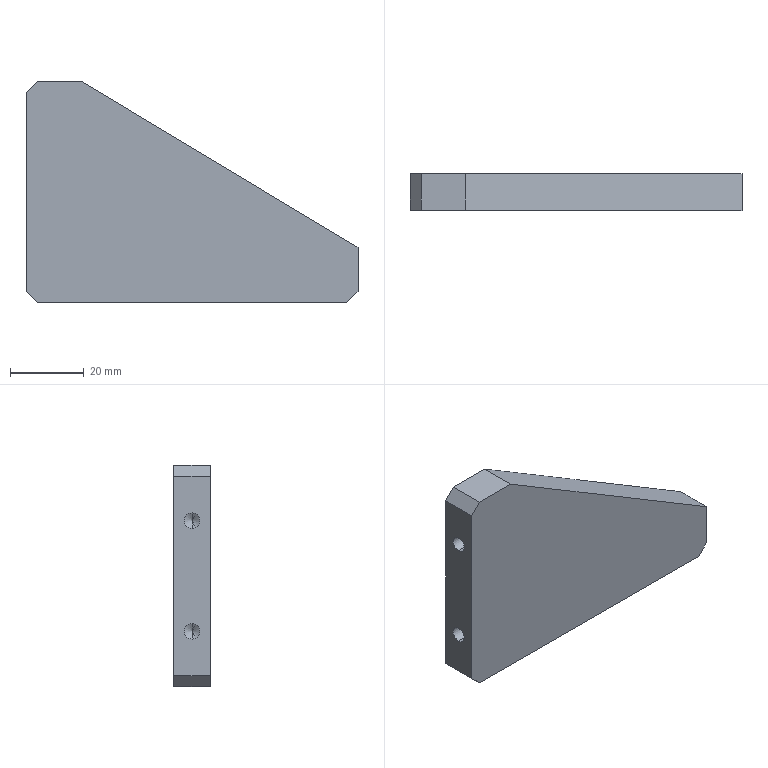Part | SolidWorks | features HoleWzd 2, Chamfer 1, Extrusion 1, ICE 1 | 1 solid | 30 faces | box 90 x 10 x 60 mm | volume 36102 mm3 | cylinder 10 | cone 10 | plane 10 | commonest cylinder face diameters 4.2 x10
STEP:
#1=CARTESIAN_POINT('',(-27.9,5.,-17.6));
#2=VERTEX_POINT('',#1);
#3=CARTESIAN_POINT('',(-32.1,5.,-17.6));
#4=VERTEX_POINT('',#3);
#5=CARTESIAN_POINT('',(-30.,5.,-17.6));
#6=DIRECTION('',(0.,0.,-1.));
#7=DIRECTION('',(-1.,0.,0.));
#8=AXIS2_PLACEMENT_3D('',#5,#6,#7);
#9=CIRCLE('',#8,2.1);
#10=EDGE_CURVE('',#2,#4,#9,.T.);
#11=ORIENTED_EDGE('',*,*,#10,.F.);
#12=CARTESIAN_POINT('',(-27.9,5.,-30.));
#13=VERTEX_POINT('',#12);
#14=CARTESIAN_POINT('',(-27.9,5.,-30.));
#15=DIRECTION('',(0.,0.,-1.));
#16=VECTOR('',#15,1000.);
#17=LINE('',#14,#16);
#18=EDGE_CURVE('',#2,#13,#17,.T.);
#19=ORIENTED_EDGE('',*,*,#18,.T.);
#20=CARTESIAN_POINT('',(-32.1,5.,-30.));
#21=VERTEX_POINT('',#20);
#22=CARTESIAN_POINT('',(-30.,5.,-30.));
#23=DIRECTION('',(0.,0.,-1.));
#24=DIRECTION('',(-1.,0.,0.));
#25=AXIS2_PLACEMENT_3D('',#22,#23,#24);
#26=CIRCLE('',#25,2.1);
#27=EDGE_CURVE('',#13,#21,#26,.T.);
#28=ORIENTED_EDGE('',*,*,#27,.T.);
#29=CARTESIAN_POINT('',(-32.1,5.,-30.));
#30=DIRECTION('',(0.,0.,-1.));
#31=VECTOR('',#30,1000.);
#32=LINE('',#29,#31);
#33=EDGE_CURVE('',#4,#21,#32,.T.);
#34=ORIENTED_EDGE('',*,*,#33,.F.);
#35=EDGE_LOOP('',(#11,#19,#28,#34));
#36=FACE_OUTER_BOUND('',#35,.T.);
#37=CARTESIAN_POINT('',(-30.,5.,-30.));
#38=DIRECTION('',(0.,0.,-1.));
#39=DIRECTION('',(-1.,0.,0.));
#40=AXIS2_PLACEMENT_3D('',#37,#38,#39);
#41=CYLINDRICAL_SURFACE('',#40,2.1);
#42=ADVANCED_FACE('',(#36),#41,.F.);
#43=CARTESIAN_POINT('',(-30.,5.,-16.338));
#44=VERTEX_POINT('',#43);
#45=CARTESIAN_POINT('',(-32.1,5.,-17.6));
#46=DIRECTION('',(-0.8572,0.,-0.515));
#47=VECTOR('',#46,1000.);
#48=LINE('',#45,#47);
#49=EDGE_CURVE('',#44,#4,#48,.T.);
#50=ORIENTED_EDGE('',*,*,#49,.F.);
#51=CARTESIAN_POINT('',(-27.9,5.,-17.6));
#52=DIRECTION('',(0.8572,0.,-0.515));
#53=VECTOR('',#52,1000.);
#54=LINE('',#51,#53);
#55=EDGE_CURVE('',#44,#2,#54,.T.);
#56=ORIENTED_EDGE('',*,*,#55,.T.);
#57=ORIENTED_EDGE('',*,*,#10,.T.);
#58=EDGE_LOOP('',(#50,#56,#57));
#59=FACE_OUTER_BOUND('',#58,.T.);
#60=CARTESIAN_POINT('',(-30.,5.,-17.6));
#61=DIRECTION('',(0.,0.,-1.));
#62=DIRECTION('',(-1.,0.,0.));
#63=AXIS2_PLACEMENT_3D('',#60,#61,#62);
#64=CONICAL_SURFACE('',#63,2.1,1.03);
#65=ADVANCED_FACE('',(#59),#64,.F.);
#66=CARTESIAN_POINT('',(2.1,5.,-17.6));
#67=VERTEX_POINT('',#66);
#68=CARTESIAN_POINT('',(-2.1,5.,-17.6));
#69=VERTEX_POINT('',#68);
#70=CARTESIAN_POINT('',(0.,5.,-17.6));
#71=DIRECTION('',(0.,0.,-1.));
#72=DIRECTION('',(-1.,0.,0.));
#73=AXIS2_PLACEMENT_3D('',#70,#71,#72);
#74=CIRCLE('',#73,2.1);
#75=EDGE_CURVE('',#67,#69,#74,.T.);
#76=ORIENTED_EDGE('',*,*,#75,.F.);
#77=CARTESIAN_POINT('',(2.1,5.,-30.));
#78=VERTEX_POINT('',#77);
#79=CARTESIAN_POINT('',(2.1,5.,-30.));
#80=DIRECTION('',(0.,0.,-1.));
#81=VECTOR('',#80,1000.);
#82=LINE('',#79,#81);
#83=EDGE_CURVE('',#67,#78,#82,.T.);
#84=ORIENTED_EDGE('',*,*,#83,.T.);
#85=CARTESIAN_POINT('',(-2.1,5.,-30.));
#86=VERTEX_POINT('',#85);
#87=CARTESIAN_POINT('',(0.,5.,-30.));
#88=DIRECTION('',(0.,0.,-1.));
#89=DIRECTION('',(-1.,0.,0.));
#90=AXIS2_PLACEMENT_3D('',#87,#88,#89);
#91=CIRCLE('',#90,2.1);
#92=EDGE_CURVE('',#78,#86,#91,.T.);
#93=ORIENTED_EDGE('',*,*,#92,.T.);
#94=CARTESIAN_POINT('',(-2.1,5.,-30.));
#95=DIRECTION('',(0.,0.,-1.));
#96=VECTOR('',#95,1000.);
#97=LINE('',#94,#96);
#98=EDGE_CURVE('',#69,#86,#97,.T.);
#99=ORIENTED_EDGE('',*,*,#98,.F.);
#100=EDGE_LOOP('',(#76,#84,#93,#99));
#101=FACE_OUTER_BOUND('',#100,.T.);
#102=CARTESIAN_POINT('',(0.,5.,-30.));
#103=DIRECTION('',(0.,0.,-1.));
#104=DIRECTION('',(-1.,0.,0.));
#105=AXIS2_PLACEMENT_3D('',#102,#103,#104);
#106=CYLINDRICAL_SURFACE('',#105,2.1);
#107=ADVANCED_FACE('',(#101),#106,.F.);
#108=CARTESIAN_POINT('',(0.,5.,-16.338));
#109=VERTEX_POINT('',#108);
#110=CARTESIAN_POINT('',(-2.1,5.,-17.6));
#111=DIRECTION('',(-0.8572,0.,-0.515));
#112=VECTOR('',#111,1000.);
#113=LINE('',#110,#112);
#114=EDGE_CURVE('',#109,#69,#113,.T.);
#115=ORIENTED_EDGE('',*,*,#114,.F.);
#116=CARTESIAN_POINT('',(2.1,5.,-17.6));
#117=DIRECTION('',(0.8572,0.,-0.515));
#118=VECTOR('',#117,1000.);
#119=LINE('',#116,#118);
#120=EDGE_CURVE('',#109,#67,#119,.T.);
#121=ORIENTED_EDGE('',*,*,#120,.T.);
#122=ORIENTED_EDGE('',*,*,#75,.T.);
#123=EDGE_LOOP('',(#115,#121,#122));
#124=FACE_OUTER_BOUND('',#123,.T.);
#125=CARTESIAN_POINT('',(0.,5.,-17.6));
#126=DIRECTION('',(0.,0.,-1.));
#127=DIRECTION('',(-1.,0.,0.));
#128=AXIS2_PLACEMENT_3D('',#125,#126,#127);
#129=CONICAL_SURFACE('',#128,2.1,1.03);
#130=ADVANCED_FACE('',(#124),#129,.F.);
#131=CARTESIAN_POINT('',(32.1,5.,-17.6));
#132=VERTEX_POINT('',#131);
#133=CARTESIAN_POINT('',(27.9,5.,-17.6));
#134=VERTEX_POINT('',#133);
#135=CARTESIAN_POINT('',(30.,5.,-17.6));
#136=DIRECTION('',(0.,0.,-1.));
#137=DIRECTION('',(-1.,0.,0.));
#138=AXIS2_PLACEMENT_3D('',#135,#136,#137);
#139=CIRCLE('',#138,2.1);
#140=EDGE_CURVE('',#132,#134,#139,.T.);
#141=ORIENTED_EDGE('',*,*,#140,.F.);
#142=CARTESIAN_POINT('',(32.1,5.,-30.));
#143=VERTEX_POINT('',#142);
#144=CARTESIAN_POINT('',(32.1,5.,-30.));
#145=DIRECTION('',(0.,0.,-1.));
#146=VECTOR('',#145,1000.);
#147=LINE('',#144,#146);
#148=EDGE_CURVE('',#132,#143,#147,.T.);
#149=ORIENTED_EDGE('',*,*,#148,.T.);
#150=CARTESIAN_POINT('',(27.9,5.,-30.));
#151=VERTEX_POINT('',#150);
#152=CARTESIAN_POINT('',(30.,5.,-30.));
#153=DIRECTION('',(0.,0.,-1.));
#154=DIRECTION('',(-1.,0.,0.));
#155=AXIS2_PLACEMENT_3D('',#152,#153,#154);
#156=CIRCLE('',#155,2.1);
#157=EDGE_CURVE('',#143,#151,#156,.T.);
#158=ORIENTED_EDGE('',*,*,#157,.T.);
#159=CARTESIAN_POINT('',(27.9,5.,-30.));
#160=DIRECTION('',(0.,0.,-1.));
#161=VECTOR('',#160,1000.);
#162=LINE('',#159,#161);
#163=EDGE_CURVE('',#134,#151,#162,.T.);
#164=ORIENTED_EDGE('',*,*,#163,.F.);
#165=EDGE_LOOP('',(#141,#149,#158,#164));
#166=FACE_OUTER_BOUND('',#165,.T.);
#167=CARTESIAN_POINT('',(30.,5.,-30.));
#168=DIRECTION('',(0.,0.,-1.));
#169=DIRECTION('',(-1.,0.,0.));
#170=AXIS2_PLACEMENT_3D('',#167,#168,#169);
#171=CYLINDRICAL_SURFACE('',#170,2.1);
#172=ADVANCED_FACE('',(#166),#171,.F.);
#173=CARTESIAN_POINT('',(30.,5.,-16.338));
#174=VERTEX_POINT('',#173);
#175=CARTESIAN_POINT('',(27.9,5.,-17.6));
#176=DIRECTION('',(-0.8572,0.,-0.515));
#177=VECTOR('',#176,1000.);
#178=LINE('',#175,#177);
#179=EDGE_CURVE('',#174,#134,#178,.T.);
#180=ORIENTED_EDGE('',*,*,#179,.F.);
#181=CARTESIAN_POINT('',(32.1,5.,-17.6));
#182=DIRECTION('',(0.8572,0.,-0.515));
#183=VECTOR('',#182,1000.);
#184=LINE('',#181,#183);
#185=EDGE_CURVE('',#174,#132,#184,.T.);
#186=ORIENTED_EDGE('',*,*,#185,.T.);
#187=ORIENTED_EDGE('',*,*,#140,.T.);
#188=EDGE_LOOP('',(#180,#186,#187));
#189=FACE_OUTER_BOUND('',#188,.T.);
#190=CARTESIAN_POINT('',(30.,5.,-17.6));
#191=DIRECTION('',(0.,0.,-1.));
#192=DIRECTION('',(-1.,0.,0.));
#193=AXIS2_PLACEMENT_3D('',#190,#191,#192);
#194=CONICAL_SURFACE('',#193,2.1,1.03);
#195=ADVANCED_FACE('',(#189),#194,.F.);
#196=CARTESIAN_POINT('',(-32.6,5.,-17.1));
#197=VERTEX_POINT('',#196);
#198=CARTESIAN_POINT('',(-32.6,5.,-12.9));
#199=VERTEX_POINT('',#198);
#200=CARTESIAN_POINT('',(-32.6,5.,-15.));
#201=DIRECTION('',(-1.,0.,0.));
#202=DIRECTION('',(0.,0.,1.));
#203=AXIS2_PLACEMENT_3D('',#200,#201,#202);
#204=CIRCLE('',#203,2.1);
#205=EDGE_CURVE('',#197,#199,#204,.T.);
#206=ORIENTED_EDGE('',*,*,#205,.F.);
#207=CARTESIAN_POINT('',(-45.,5.,-17.1));
#208=VERTEX_POINT('',#207);
#209=CARTESIAN_POINT('',(-45.,5.,-17.1));
#210=DIRECTION('',(-1.,0.,0.));
#211=VECTOR('',#210,1000.);
#212=LINE('',#209,#211);
#213=EDGE_CURVE('',#197,#208,#212,.T.);
#214=ORIENTED_EDGE('',*,*,#213,.T.);
#215=CARTESIAN_POINT('',(-45.,5.,-12.9));
#216=VERTEX_POINT('',#215);
#217=CARTESIAN_POINT('',(-45.,5.,-15.));
#218=DIRECTION('',(-1.,0.,0.));
#219=DIRECTION('',(0.,0.,1.));
#220=AXIS2_PLACEMENT_3D('',#217,#218,#219);
#221=CIRCLE('',#220,2.1);
#222=EDGE_CURVE('',#208,#216,#221,.T.);
#223=ORIENTED_EDGE('',*,*,#222,.T.);
#224=CARTESIAN_POINT('',(-45.,5.,-12.9));
#225=DIRECTION('',(-1.,0.,0.));
#226=VECTOR('',#225,1000.);
#227=LINE('',#224,#226);
#228=EDGE_CURVE('',#199,#216,#227,.T.);
#229=ORIENTED_EDGE('',*,*,#228,.F.);
#230=EDGE_LOOP('',(#206,#214,#223,#229));
#231=FACE_OUTER_BOUND('',#230,.T.);
#232=CARTESIAN_POINT('',(-45.,5.,-15.));
#233=DIRECTION('',(-1.,0.,0.));
#234=DIRECTION('',(0.,0.,1.));
#235=AXIS2_PLACEMENT_3D('',#232,#233,#234);
#236=CYLINDRICAL_SURFACE('',#235,2.1);
#237=ADVANCED_FACE('',(#231),#236,.F.);
#238=CARTESIAN_POINT('',(-31.338,5.,-15.));
#239=VERTEX_POINT('',#238);
#240=CARTESIAN_POINT('',(-32.6,5.,-12.9));
#241=DIRECTION('',(-0.515,0.,0.8572));
#242=VECTOR('',#241,1000.);
#243=LINE('',#240,#242);
#244=EDGE_CURVE('',#239,#199,#243,.T.);
#245=ORIENTED_EDGE('',*,*,#244,.F.);
#246=CARTESIAN_POINT('',(-32.6,5.,-17.1));
#247=DIRECTION('',(-0.515,0.,-0.8572));
#248=VECTOR('',#247,1000.);
#249=LINE('',#246,#248);
#250=EDGE_CURVE('',#239,#197,#249,.T.);
#251=ORIENTED_EDGE('',*,*,#250,.T.);
#252=ORIENTED_EDGE('',*,*,#205,.T.);
#253=EDGE_LOOP('',(#245,#251,#252));
#254=FACE_OUTER_BOUND('',#253,.T.);
#255=CARTESIAN_POINT('',(-32.6,5.,-15.));
#256=DIRECTION('',(-1.,0.,0.));
#257=DIRECTION('',(0.,0.,1.));
#258=AXIS2_PLACEMENT_3D('',#255,#256,#257);
#259=CONICAL_SURFACE('',#258,2.1,1.03);
#260=ADVANCED_FACE('',(#254),#259,.F.);
#261=CARTESIAN_POINT('',(-32.6,5.,12.9));
#262=VERTEX_POINT('',#261);
#263=CARTESIAN_POINT('',(-32.6,5.,17.1));
#264=VERTEX_POINT('',#263);
#265=CARTESIAN_POINT('',(-32.6,5.,15.));
#266=DIRECTION('',(-1.,0.,0.));
#267=DIRECTION('',(0.,0.,1.));
#268=AXIS2_PLACEMENT_3D('',#265,#266,#267);
#269=CIRCLE('',#268,2.1);
#270=EDGE_CURVE('',#262,#264,#269,.T.);
#271=ORIENTED_EDGE('',*,*,#270,.F.);
#272=CARTESIAN_POINT('',(-45.,5.,12.9));
#273=VERTEX_POINT('',#272);
#274=CARTESIAN_POINT('',(-45.,5.,12.9));
#275=DIRECTION('',(-1.,0.,0.));
#276=VECTOR('',#275,1000.);
#277=LINE('',#274,#276);
#278=EDGE_CURVE('',#262,#273,#277,.T.);
#279=ORIENTED_EDGE('',*,*,#278,.T.);
#280=CARTESIAN_POINT('',(-45.,5.,17.1));
#281=VERTEX_POINT('',#280);
#282=CARTESIAN_POINT('',(-45.,5.,15.));
#283=DIRECTION('',(-1.,0.,0.));
#284=DIRECTION('',(0.,0.,1.));
#285=AXIS2_PLACEMENT_3D('',#282,#283,#284);
#286=CIRCLE('',#285,2.1);
#287=EDGE_CURVE('',#273,#281,#286,.T.);
#288=ORIENTED_EDGE('',*,*,#287,.T.);
#289=CARTESIAN_POINT('',(-45.,5.,17.1));
#290=DIRECTION('',(-1.,0.,0.));
#291=VECTOR('',#290,1000.);
#292=LINE('',#289,#291);
#293=EDGE_CURVE('',#264,#281,#292,.T.);
#294=ORIENTED_EDGE('',*,*,#293,.F.);
#295=EDGE_LOOP('',(#271,#279,#288,#294));
#296=FACE_OUTER_BOUND('',#295,.T.);
#297=CARTESIAN_POINT('',(-45.,5.,15.));
#298=DIRECTION('',(-1.,0.,0.));
#299=DIRECTION('',(0.,0.,1.));
#300=AXIS2_PLACEMENT_3D('',#297,#298,#299);
#301=CYLINDRICAL_SURFACE('',#300,2.1);
#302=ADVANCED_FACE('',(#296),#301,.F.);
#303=CARTESIAN_POINT('',(-31.338,5.,15.));
#304=VERTEX_POINT('',#303);
#305=CARTESIAN_POINT('',(-32.6,5.,17.1));
#306=DIRECTION('',(-0.515,0.,0.8572));
#307=VECTOR('',#306,1000.);
#308=LINE('',#305,#307);
#309=EDGE_CURVE('',#304,#264,#308,.T.);
#310=ORIENTED_EDGE('',*,*,#309,.F.);
#311=CARTESIAN_POINT('',(-32.6,5.,12.9));
#312=DIRECTION('',(-0.515,0.,-0.8572));
#313=VECTOR('',#312,1000.);
#314=LINE('',#311,#313);
#315=EDGE_CURVE('',#304,#262,#314,.T.);
#316=ORIENTED_EDGE('',*,*,#315,.T.);
#317=ORIENTED_EDGE('',*,*,#270,.T.);
#318=EDGE_LOOP('',(#310,#316,#317));
#319=FACE_OUTER_BOUND('',#318,.T.);
#320=CARTESIAN_POINT('',(-32.6,5.,15.));
#321=DIRECTION('',(-1.,0.,0.));
#322=DIRECTION('',(0.,0.,1.));
#323=AXIS2_PLACEMENT_3D('',#320,#321,#322);
#324=CONICAL_SURFACE('',#323,2.1,1.03);
#325=ADVANCED_FACE('',(#319),#324,.F.);
#326=CARTESIAN_POINT('',(45.,0.,-15.));
#327=VERTEX_POINT('',#326);
#328=CARTESIAN_POINT('',(45.,0.,-27.));
#329=VERTEX_POINT('',#328);
#330=CARTESIAN_POINT('',(45.,0.,-30.));
#331=DIRECTION('',(0.,0.,-1.));
#332=VECTOR('',#331,1000.);
#333=LINE('',#330,#332);
#334=EDGE_CURVE('',#327,#329,#333,.T.);
#335=ORIENTED_EDGE('',*,*,#334,.T.);
#336=CARTESIAN_POINT('',(45.,10.,-27.));
#337=VERTEX_POINT('',#336);
#338=CARTESIAN_POINT('',(45.,10.,-27.));
#339=DIRECTION('',(0.,1.,0.));
#340=VECTOR('',#339,1000.);
#341=LINE('',#338,#340);
#342=EDGE_CURVE('',#329,#337,#341,.T.);
#343=ORIENTED_EDGE('',*,*,#342,.T.);
#344=CARTESIAN_POINT('',(45.,10.,-15.));
#345=VERTEX_POINT('',#344);
#346=CARTESIAN_POINT('',(45.,10.,-30.));
#347=DIRECTION('',(0.,0.,-1.));
#348=VECTOR('',#347,1000.);
#349=LINE('',#346,#348);
#350=EDGE_CURVE('',#345,#337,#349,.T.);
#351=ORIENTED_EDGE('',*,*,#350,.F.);
#352=CARTESIAN_POINT('',(45.,-5.,-15.));
#353=DIRECTION('',(0.,1.,0.));
#354=VECTOR('',#353,1000.);
#355=LINE('',#352,#354);
#356=EDGE_CURVE('',#327,#345,#355,.T.);
#357=ORIENTED_EDGE('',*,*,#356,.F.);
#358=EDGE_LOOP('',(#335,#343,#351,#357));
#359=FACE_OUTER_BOUND('',#358,.T.);
#360=CARTESIAN_POINT('',(45.,10.,-30.));
#361=DIRECTION('',(-1.,0.,0.));
#362=DIRECTION('',(0.,0.,1.));
#363=AXIS2_PLACEMENT_3D('',#360,#361,#362);
#364=PLANE('',#363);
#365=ADVANCED_FACE('',(#359),#364,.F.);
#366=CARTESIAN_POINT('',(-30.,5.,-30.));
#367=DIRECTION('',(0.,0.,-1.));
#368=DIRECTION('',(-1.,0.,0.));
#369=AXIS2_PLACEMENT_3D('',#366,#367,#368);
#370=CIRCLE('',#369,2.1);
#371=EDGE_CURVE('',#21,#13,#370,.T.);
#372=ORIENTED_EDGE('',*,*,#371,.F.);
#373=ORIENTED_EDGE('',*,*,#27,.F.);
#374=EDGE_LOOP('',(#372,#373));
#375=FACE_BOUND('',#374,.T.);
#376=CARTESIAN_POINT('',(0.,5.,-30.));
#377=DIRECTION('',(0.,0.,-1.));
#378=DIRECTION('',(-1.,0.,0.));
#379=AXIS2_PLACEMENT_3D('',#376,#377,#378);
#380=CIRCLE('',#379,2.1);
#381=EDGE_CURVE('',#86,#78,#380,.T.);
#382=ORIENTED_EDGE('',*,*,#381,.F.);
#383=ORIENTED_EDGE('',*,*,#92,.F.);
#384=EDGE_LOOP('',(#382,#383));
#385=FACE_BOUND('',#384,.T.);
#386=CARTESIAN_POINT('',(30.,5.,-30.));
#387=DIRECTION('',(0.,0.,-1.));
#388=DIRECTION('',(-1.,0.,0.));
#389=AXIS2_PLACEMENT_3D('',#386,#387,#388);
#390=CIRCLE('',#389,2.1);
#391=EDGE_CURVE('',#151,#143,#390,.T.);
#392=ORIENTED_EDGE('',*,*,#391,.F.);
#393=ORIENTED_EDGE('',*,*,#157,.F.);
#394=EDGE_LOOP('',(#392,#393));
#395=FACE_BOUND('',#394,.T.);
#396=CARTESIAN_POINT('',(42.,10.,-30.));
#397=VERTEX_POINT('',#396);
#398=CARTESIAN_POINT('',(-42.,10.,-30.));
#399=VERTEX_POINT('',#398);
#400=CARTESIAN_POINT('',(-45.,10.,-30.));
#401=DIRECTION('',(-1.,0.,0.));
#402=VECTOR('',#401,1000.);
#403=LINE('',#400,#402);
#404=EDGE_CURVE('',#397,#399,#403,.T.);
#405=ORIENTED_EDGE('',*,*,#404,.F.);
#406=CARTESIAN_POINT('',(42.,0.,-30.));
#407=VERTEX_POINT('',#406);
#408=CARTESIAN_POINT('',(42.,10.,-30.));
#409=DIRECTION('',(0.,-1.,0.));
#410=VECTOR('',#409,1000.);
#411=LINE('',#408,#410);
#412=EDGE_CURVE('',#397,#407,#411,.T.);
#413=ORIENTED_EDGE('',*,*,#412,.T.);
#414=CARTESIAN_POINT('',(-42.,0.,-30.));
#415=VERTEX_POINT('',#414);
#416=CARTESIAN_POINT('',(-45.,0.,-30.));
#417=DIRECTION('',(-1.,0.,0.));
#418=VECTOR('',#417,1000.);
#419=LINE('',#416,#418);
#420=EDGE_CURVE('',#407,#415,#419,.T.);
#421=ORIENTED_EDGE('',*,*,#420,.T.);
#422=CARTESIAN_POINT('',(-42.,10.,-30.));
#423=DIRECTION('',(0.,1.,0.));
#424=VECTOR('',#423,1000.);
#425=LINE('',#422,#424);
#426=EDGE_CURVE('',#415,#399,#425,.T.);
#427=ORIENTED_EDGE('',*,*,#426,.T.);
#428=EDGE_LOOP('',(#405,#413,#421,#427));
#429=FACE_OUTER_BOUND('',#428,.T.);
#430=CARTESIAN_POINT('',(-45.,10.,-30.));
#431=DIRECTION('',(0.,0.,1.));
#432=DIRECTION('',(1.,0.,0.));
#433=AXIS2_PLACEMENT_3D('',#430,#431,#432);
#434=PLANE('',#433);
#435=ADVANCED_FACE('',(#375,#385,#395,#429),#434,.F.);
#436=CARTESIAN_POINT('',(-45.,5.,-15.));
#437=DIRECTION('',(-1.,0.,0.));
#438=DIRECTION('',(0.,0.,1.));
#439=AXIS2_PLACEMENT_3D('',#436,#437,#438);
#440=CIRCLE('',#439,2.1);
#441=EDGE_CURVE('',#216,#208,#440,.T.);
#442=ORIENTED_EDGE('',*,*,#441,.F.);
#443=ORIENTED_EDGE('',*,*,#222,.F.);
#444=EDGE_LOOP('',(#442,#443));
#445=FACE_BOUND('',#444,.T.);
#446=CARTESIAN_POINT('',(-45.,5.,15.));
#447=DIRECTION('',(-1.,0.,0.));
#448=DIRECTION('',(0.,0.,1.));
#449=AXIS2_PLACEMENT_3D('',#446,#447,#448);
#450=CIRCLE('',#449,2.1);
#451=EDGE_CURVE('',#281,#273,#450,.T.);
#452=ORIENTED_EDGE('',*,*,#451,.F.);
#453=ORIENTED_EDGE('',*,*,#287,.F.);
#454=EDGE_LOOP('',(#452,#453));
#455=FACE_BOUND('',#454,.T.);
#456=CARTESIAN_POINT('',(-45.,0.,-27.));
#457=VERTEX_POINT('',#456);
#458=CARTESIAN_POINT('',(-45.,0.,27.));
#459=VERTEX_POINT('',#458);
#460=CARTESIAN_POINT('',(-45.,0.,-30.));
#461=DIRECTION('',(0.,0.,1.));
#462=VECTOR('',#461,1000.);
#463=LINE('',#460,#462);
#464=EDGE_CURVE('',#457,#459,#463,.T.);
#465=ORIENTED_EDGE('',*,*,#464,.T.);
#466=CARTESIAN_POINT('',(-45.,10.,27.));
#467=VERTEX_POINT('',#466);
#468=CARTESIAN_POINT('',(-45.,10.,27.));
#469=DIRECTION('',(0.,1.,0.));
#470=VECTOR('',#469,1000.);
#471=LINE('',#468,#470);
#472=EDGE_CURVE('',#459,#467,#471,.T.);
#473=ORIENTED_EDGE('',*,*,#472,.T.);
#474=CARTESIAN_POINT('',(-45.,10.,-27.));
#475=VERTEX_POINT('',#474);
#476=CARTESIAN_POINT('',(-45.,10.,-30.));
#477=DIRECTION('',(0.,0.,1.));
#478=VECTOR('',#477,1000.);
#479=LINE('',#476,#478);
#480=EDGE_CURVE('',#475,#467,#479,.T.);
#481=ORIENTED_EDGE('',*,*,#480,.F.);
#482=CARTESIAN_POINT('',(-45.,10.,-27.));
#483=DIRECTION('',(0.,-1.,0.));
#484=VECTOR('',#483,1000.);
#485=LINE('',#482,#484);
#486=EDGE_CURVE('',#475,#457,#485,.T.);
#487=ORIENTED_EDGE('',*,*,#486,.T.);
#488=EDGE_LOOP('',(#465,#473,#481,#487));
#489=FACE_OUTER_BOUND('',#488,.T.);
#490=CARTESIAN_POINT('',(-45.,10.,-30.));
#491=DIRECTION('',(1.,0.,0.));
#492=DIRECTION('',(0.,0.,-1.));
#493=AXIS2_PLACEMENT_3D('',#490,#491,#492);
#494=PLANE('',#493);
#495=ADVANCED_FACE('',(#445,#455,#489),#494,.F.);
#496=CARTESIAN_POINT('',(-42.,10.,30.));
#497=VERTEX_POINT('',#496);
#498=CARTESIAN_POINT('',(-30.,10.,30.));
#499=VERTEX_POINT('',#498);
#500=CARTESIAN_POINT('',(-45.,10.,30.));
#501=DIRECTION('',(1.,0.,0.));
#502=VECTOR('',#501,1000.);
#503=LINE('',#500,#502);
#504=EDGE_CURVE('',#497,#499,#503,.T.);
#505=ORIENTED_EDGE('',*,*,#504,.F.);
#506=CARTESIAN_POINT('',(-42.,0.,30.));
#507=VERTEX_POINT('',#506);
#508=CARTESIAN_POINT('',(-42.,10.,30.));
#509=DIRECTION('',(0.,-1.,0.));
#510=VECTOR('',#509,1000.);
#511=LINE('',#508,#510);
#512=EDGE_CURVE('',#497,#507,#511,.T.);
#513=ORIENTED_EDGE('',*,*,#512,.T.);
#514=CARTESIAN_POINT('',(-30.,0.,30.));
#515=VERTEX_POINT('',#514);
#516=CARTESIAN_POINT('',(-45.,0.,30.));
#517=DIRECTION('',(1.,0.,0.));
#518=VECTOR('',#517,1000.);
#519=LINE('',#516,#518);
#520=EDGE_CURVE('',#507,#515,#519,.T.);
#521=ORIENTED_EDGE('',*,*,#520,.T.);
#522=CARTESIAN_POINT('',(-30.,-5.,30.));
#523=DIRECTION('',(0.,1.,0.));
#524=VECTOR('',#523,1000.);
#525=LINE('',#522,#524);
#526=EDGE_CURVE('',#515,#499,#525,.T.);
#527=ORIENTED_EDGE('',*,*,#526,.T.);
#528=EDGE_LOOP('',(#505,#513,#521,#527));
#529=FACE_OUTER_BOUND('',#528,.T.);
#530=CARTESIAN_POINT('',(-45.,10.,30.));
#531=DIRECTION('',(0.,0.,-1.));
#532=DIRECTION('',(-1.,0.,0.));
#533=AXIS2_PLACEMENT_3D('',#530,#531,#532);
#534=PLANE('',#533);
#535=ADVANCED_FACE('',(#529),#534,.F.);
#536=ORIENTED_EDGE('',*,*,#350,.T.);
#537=CARTESIAN_POINT('',(36.,10.,-36.));
#538=DIRECTION('',(-0.7071,0.,-0.7071));
#539=VECTOR('',#538,1000.);
#540=LINE('',#537,#539);
#541=EDGE_CURVE('',#337,#397,#540,.T.);
#542=ORIENTED_EDGE('',*,*,#541,.T.);
#543=ORIENTED_EDGE('',*,*,#404,.T.);
#544=CARTESIAN_POINT('',(-36.,10.,-36.));
#545=DIRECTION('',(-0.7071,0.,0.7071));
#546=VECTOR('',#545,1000.);
#547=LINE('',#544,#546);
#548=EDGE_CURVE('',#399,#475,#547,.T.);
#549=ORIENTED_EDGE('',*,*,#548,.T.);
#550=ORIENTED_EDGE('',*,*,#480,.T.);
#551=CARTESIAN_POINT('',(-36.,10.,36.));
#552=DIRECTION('',(0.7071,0.,0.7071));
#553=VECTOR('',#552,1000.);
#554=LINE('',#551,#553);
#555=EDGE_CURVE('',#467,#497,#554,.T.);
#556=ORIENTED_EDGE('',*,*,#555,.T.);
#557=ORIENTED_EDGE('',*,*,#504,.T.);
#558=CARTESIAN_POINT('',(45.,10.,-15.));
#559=DIRECTION('',(-0.8575,0.,0.5145));
#560=VECTOR('',#559,1000.);
#561=LINE('',#558,#560);
#562=EDGE_CURVE('',#345,#499,#561,.T.);
#563=ORIENTED_EDGE('',*,*,#562,.F.);
#564=EDGE_LOOP('',(#536,#542,#543,#549,#550,#556,#557,#563));
#565=FACE_OUTER_BOUND('',#564,.T.);
#566=CARTESIAN_POINT('',(0.,10.,0.));
#567=DIRECTION('',(0.,1.,0.));
#568=DIRECTION('',(0.,0.,1.));
#569=AXIS2_PLACEMENT_3D('',#566,#567,#568);
#570=PLANE('',#569);
#571=ADVANCED_FACE('',(#565),#570,.T.);
#572=ORIENTED_EDGE('',*,*,#420,.F.);
#573=CARTESIAN_POINT('',(42.,0.,-30.));
#574=DIRECTION('',(0.7071,0.,0.7071));
#575=VECTOR('',#574,1000.);
#576=LINE('',#573,#575);
#577=EDGE_CURVE('',#407,#329,#576,.T.);
#578=ORIENTED_EDGE('',*,*,#577,.T.);
#579=ORIENTED_EDGE('',*,*,#334,.F.);
#580=CARTESIAN_POINT('',(5.294,0.,8.824));
#581=DIRECTION('',(-0.8575,0.,0.5145));
#582=VECTOR('',#581,1000.);
#583=LINE('',#580,#582);
#584=EDGE_CURVE('',#327,#515,#583,.T.);
#585=ORIENTED_EDGE('',*,*,#584,.T.);
#586=ORIENTED_EDGE('',*,*,#520,.F.);
#587=CARTESIAN_POINT('',(-42.,0.,30.));
#588=DIRECTION('',(-0.7071,0.,-0.7071));
#589=VECTOR('',#588,1000.);
#590=LINE('',#587,#589);
#591=EDGE_CURVE('',#507,#459,#590,.T.);
#592=ORIENTED_EDGE('',*,*,#591,.T.);
#593=ORIENTED_EDGE('',*,*,#464,.F.);
#594=CARTESIAN_POINT('',(-45.,0.,-27.));
#595=DIRECTION('',(0.7071,0.,-0.7071));
#596=VECTOR('',#595,1000.);
#597=LINE('',#594,#596);
#598=EDGE_CURVE('',#457,#415,#597,.T.);
#599=ORIENTED_EDGE('',*,*,#598,.T.);
#600=EDGE_LOOP('',(#572,#578,#579,#585,#586,#592,#593,#599));
#601=FACE_OUTER_BOUND('',#600,.T.);
#602=CARTESIAN_POINT('',(0.,0.,0.));
#603=DIRECTION('',(0.,1.,0.));
#604=DIRECTION('',(0.,0.,1.));
#605=AXIS2_PLACEMENT_3D('',#602,#603,#604);
#606=PLANE('',#605);
#607=ADVANCED_FACE('',(#601),#606,.F.);
#608=ORIENTED_EDGE('',*,*,#356,.T.);
#609=ORIENTED_EDGE('',*,*,#562,.T.);
#610=ORIENTED_EDGE('',*,*,#526,.F.);
#611=ORIENTED_EDGE('',*,*,#584,.F.);
#612=EDGE_LOOP('',(#608,#609,#610,#611));
#613=FACE_OUTER_BOUND('',#612,.T.);
#614=CARTESIAN_POINT('',(45.,-5.,-15.));
#615=DIRECTION('',(-0.5145,0.,-0.8575));
#616=DIRECTION('',(-0.8575,0.,0.5145));
#617=AXIS2_PLACEMENT_3D('',#614,#615,#616);
#618=PLANE('',#617);
#619=ADVANCED_FACE('',(#613),#618,.F.);
#620=ORIENTED_EDGE('',*,*,#541,.F.);
#621=ORIENTED_EDGE('',*,*,#342,.F.);
#622=ORIENTED_EDGE('',*,*,#577,.F.);
#623=ORIENTED_EDGE('',*,*,#412,.F.);
#624=EDGE_LOOP('',(#620,#621,#622,#623));
#625=FACE_OUTER_BOUND('',#624,.T.);
#626=CARTESIAN_POINT('',(42.,10.,-30.));
#627=DIRECTION('',(-0.7071,0.,0.7071));
#628=DIRECTION('',(0.,-1.,0.));
#629=AXIS2_PLACEMENT_3D('',#626,#627,#628);
#630=PLANE('',#629);
#631=ADVANCED_FACE('',(#625),#630,.F.);
#632=ORIENTED_EDGE('',*,*,#555,.F.);
#633=ORIENTED_EDGE('',*,*,#472,.F.);
#634=ORIENTED_EDGE('',*,*,#591,.F.);
#635=ORIENTED_EDGE('',*,*,#512,.F.);
#636=EDGE_LOOP('',(#632,#633,#634,#635));
#637=FACE_OUTER_BOUND('',#636,.T.);
#638=CARTESIAN_POINT('',(-42.,10.,30.));
#639=DIRECTION('',(0.7071,0.,-0.7071));
#640=DIRECTION('',(0.,-1.,0.));
#641=AXIS2_PLACEMENT_3D('',#638,#639,#640);
#642=PLANE('',#641);
#643=ADVANCED_FACE('',(#637),#642,.F.);
#644=ORIENTED_EDGE('',*,*,#548,.F.);
#645=ORIENTED_EDGE('',*,*,#426,.F.);
#646=ORIENTED_EDGE('',*,*,#598,.F.);
#647=ORIENTED_EDGE('',*,*,#486,.F.);
#648=EDGE_LOOP('',(#644,#645,#646,#647));
#649=FACE_OUTER_BOUND('',#648,.T.);
#650=CARTESIAN_POINT('',(-45.,10.,-27.));
#651=DIRECTION('',(0.7071,0.,0.7071));
#652=DIRECTION('',(0.,-1.,0.));
#653=AXIS2_PLACEMENT_3D('',#650,#651,#652);
#654=PLANE('',#653);
#655=ADVANCED_FACE('',(#649),#654,.F.);
#656=ORIENTED_EDGE('',*,*,#315,.F.);
#657=ORIENTED_EDGE('',*,*,#309,.T.);
#658=CARTESIAN_POINT('',(-32.6,5.,15.));
#659=DIRECTION('',(-1.,0.,0.));
#660=DIRECTION('',(0.,0.,1.));
#661=AXIS2_PLACEMENT_3D('',#658,#659,#660);
#662=CIRCLE('',#661,2.1);
#663=EDGE_CURVE('',#264,#262,#662,.T.);
#664=ORIENTED_EDGE('',*,*,#663,.T.);
#665=EDGE_LOOP('',(#656,#657,#664));
#666=FACE_OUTER_BOUND('',#665,.T.);
#667=CARTESIAN_POINT('',(-32.6,5.,15.));
#668=DIRECTION('',(-1.,0.,0.));
#669=DIRECTION('',(0.,0.,1.));
#670=AXIS2_PLACEMENT_3D('',#667,#668,#669);
#671=CONICAL_SURFACE('',#670,2.1,1.03);
#672=ADVANCED_FACE('',(#666),#671,.F.);
#673=ORIENTED_EDGE('',*,*,#278,.F.);
#674=ORIENTED_EDGE('',*,*,#663,.F.);
#675=ORIENTED_EDGE('',*,*,#293,.T.);
#676=ORIENTED_EDGE('',*,*,#451,.T.);
#677=EDGE_LOOP('',(#673,#674,#675,#676));
#678=FACE_OUTER_BOUND('',#677,.T.);
#679=CARTESIAN_POINT('',(-45.,5.,15.));
#680=DIRECTION('',(-1.,0.,0.));
#681=DIRECTION('',(0.,0.,1.));
#682=AXIS2_PLACEMENT_3D('',#679,#680,#681);
#683=CYLINDRICAL_SURFACE('',#682,2.1);
#684=ADVANCED_FACE('',(#678),#683,.F.);
#685=ORIENTED_EDGE('',*,*,#250,.F.);
#686=ORIENTED_EDGE('',*,*,#244,.T.);
#687=CARTESIAN_POINT('',(-32.6,5.,-15.));
#688=DIRECTION('',(-1.,0.,0.));
#689=DIRECTION('',(0.,0.,1.));
#690=AXIS2_PLACEMENT_3D('',#687,#688,#689);
#691=CIRCLE('',#690,2.1);
#692=EDGE_CURVE('',#199,#197,#691,.T.);
#693=ORIENTED_EDGE('',*,*,#692,.T.);
#694=EDGE_LOOP('',(#685,#686,#693));
#695=FACE_OUTER_BOUND('',#694,.T.);
#696=CARTESIAN_POINT('',(-32.6,5.,-15.));
#697=DIRECTION('',(-1.,0.,0.));
#698=DIRECTION('',(0.,0.,1.));
#699=AXIS2_PLACEMENT_3D('',#696,#697,#698);
#700=CONICAL_SURFACE('',#699,2.1,1.03);
#701=ADVANCED_FACE('',(#695),#700,.F.);
#702=ORIENTED_EDGE('',*,*,#213,.F.);
#703=ORIENTED_EDGE('',*,*,#692,.F.);
#704=ORIENTED_EDGE('',*,*,#228,.T.);
#705=ORIENTED_EDGE('',*,*,#441,.T.);
#706=EDGE_LOOP('',(#702,#703,#704,#705));
#707=FACE_OUTER_BOUND('',#706,.T.);
#708=CARTESIAN_POINT('',(-45.,5.,-15.));
#709=DIRECTION('',(-1.,0.,0.));
#710=DIRECTION('',(0.,0.,1.));
#711=AXIS2_PLACEMENT_3D('',#708,#709,#710);
#712=CYLINDRICAL_SURFACE('',#711,2.1);
#713=ADVANCED_FACE('',(#707),#712,.F.);
#714=ORIENTED_EDGE('',*,*,#185,.F.);
#715=ORIENTED_EDGE('',*,*,#179,.T.);
#716=CARTESIAN_POINT('',(30.,5.,-17.6));
#717=DIRECTION('',(0.,0.,-1.));
#718=DIRECTION('',(-1.,0.,0.));
#719=AXIS2_PLACEMENT_3D('',#716,#717,#718);
#720=CIRCLE('',#719,2.1);
#721=EDGE_CURVE('',#134,#132,#720,.T.);
#722=ORIENTED_EDGE('',*,*,#721,.T.);
#723=EDGE_LOOP('',(#714,#715,#722));
#724=FACE_OUTER_BOUND('',#723,.T.);
#725=CARTESIAN_POINT('',(30.,5.,-17.6));
#726=DIRECTION('',(0.,0.,-1.));
#727=DIRECTION('',(-1.,0.,0.));
#728=AXIS2_PLACEMENT_3D('',#725,#726,#727);
#729=CONICAL_SURFACE('',#728,2.1,1.03);
#730=ADVANCED_FACE('',(#724),#729,.F.);
#731=ORIENTED_EDGE('',*,*,#148,.F.);
#732=ORIENTED_EDGE('',*,*,#721,.F.);
#733=ORIENTED_EDGE('',*,*,#163,.T.);
#734=ORIENTED_EDGE('',*,*,#391,.T.);
#735=EDGE_LOOP('',(#731,#732,#733,#734));
#736=FACE_OUTER_BOUND('',#735,.T.);
#737=CARTESIAN_POINT('',(30.,5.,-30.));
#738=DIRECTION('',(0.,0.,-1.));
#739=DIRECTION('',(-1.,0.,0.));
#740=AXIS2_PLACEMENT_3D('',#737,#738,#739);
#741=CYLINDRICAL_SURFACE('',#740,2.1);
#742=ADVANCED_FACE('',(#736),#741,.F.);
#743=ORIENTED_EDGE('',*,*,#120,.F.);
#744=ORIENTED_EDGE('',*,*,#114,.T.);
#745=CARTESIAN_POINT('',(0.,5.,-17.6));
#746=DIRECTION('',(0.,0.,-1.));
#747=DIRECTION('',(-1.,0.,0.));
#748=AXIS2_PLACEMENT_3D('',#745,#746,#747);
#749=CIRCLE('',#748,2.1);
#750=EDGE_CURVE('',#69,#67,#749,.T.);
#751=ORIENTED_EDGE('',*,*,#750,.T.);
#752=EDGE_LOOP('',(#743,#744,#751));
#753=FACE_OUTER_BOUND('',#752,.T.);
#754=CARTESIAN_POINT('',(0.,5.,-17.6));
#755=DIRECTION('',(0.,0.,-1.));
#756=DIRECTION('',(-1.,0.,0.));
#757=AXIS2_PLACEMENT_3D('',#754,#755,#756);
#758=CONICAL_SURFACE('',#757,2.1,1.03);
#759=ADVANCED_FACE('',(#753),#758,.F.);
#760=ORIENTED_EDGE('',*,*,#83,.F.);
#761=ORIENTED_EDGE('',*,*,#750,.F.);
#762=ORIENTED_EDGE('',*,*,#98,.T.);
#763=ORIENTED_EDGE('',*,*,#381,.T.);
#764=EDGE_LOOP('',(#760,#761,#762,#763));
#765=FACE_OUTER_BOUND('',#764,.T.);
#766=CARTESIAN_POINT('',(0.,5.,-30.));
#767=DIRECTION('',(0.,0.,-1.));
#768=DIRECTION('',(-1.,0.,0.));
#769=AXIS2_PLACEMENT_3D('',#766,#767,#768);
#770=CYLINDRICAL_SURFACE('',#769,2.1);
#771=ADVANCED_FACE('',(#765),#770,.F.);
#772=ORIENTED_EDGE('',*,*,#55,.F.);
#773=ORIENTED_EDGE('',*,*,#49,.T.);
#774=CARTESIAN_POINT('',(-30.,5.,-17.6));
#775=DIRECTION('',(0.,0.,-1.));
#776=DIRECTION('',(-1.,0.,0.));
#777=AXIS2_PLACEMENT_3D('',#774,#775,#776);
#778=CIRCLE('',#777,2.1);
#779=EDGE_CURVE('',#4,#2,#778,.T.);
#780=ORIENTED_EDGE('',*,*,#779,.T.);
#781=EDGE_LOOP('',(#772,#773,#780));
#782=FACE_OUTER_BOUND('',#781,.T.);
#783=CARTESIAN_POINT('',(-30.,5.,-17.6));
#784=DIRECTION('',(0.,0.,-1.));
#785=DIRECTION('',(-1.,0.,0.));
#786=AXIS2_PLACEMENT_3D('',#783,#784,#785);
#787=CONICAL_SURFACE('',#786,2.1,1.03);
#788=ADVANCED_FACE('',(#782),#787,.F.);
#789=ORIENTED_EDGE('',*,*,#18,.F.);
#790=ORIENTED_EDGE('',*,*,#779,.F.);
#791=ORIENTED_EDGE('',*,*,#33,.T.);
#792=ORIENTED_EDGE('',*,*,#371,.T.);
#793=EDGE_LOOP('',(#789,#790,#791,#792));
#794=FACE_OUTER_BOUND('',#793,.T.);
#795=CARTESIAN_POINT('',(-30.,5.,-30.));
#796=DIRECTION('',(0.,0.,-1.));
#797=DIRECTION('',(-1.,0.,0.));
#798=AXIS2_PLACEMENT_3D('',#795,#796,#797);
#799=CYLINDRICAL_SURFACE('',#798,2.1);
#800=ADVANCED_FACE('',(#794),#799,.F.);
#801=CLOSED_SHELL('',(#42,#65,#107,#130,#172,#195,#237,#260,#302,#325,#365,#435,#495,#535,#571,#607,#619,#631,#643,#655,#672,#684,#701,#713,#730,#742,#759,#771,#788,#800));
#802=MANIFOLD_SOLID_BREP('',#801);
#803=CARTESIAN_POINT('',(0.,0.,0.));
#804=DIRECTION('',(0.,0.,1.));
#805=DIRECTION('',(1.,0.,0.));
#806=AXIS2_PLACEMENT_3D('',#803,#804,#805);
#807=(LENGTH_UNIT()NAMED_UNIT(*)SI_UNIT(.MILLI.,.METRE.));
#808=UNCERTAINTY_MEASURE_WITH_UNIT(LENGTH_MEASURE(0.00001),#807,'','');
#809=(NAMED_UNIT(*)PLANE_ANGLE_UNIT()SI_UNIT($,.RADIAN.));
#810=(NAMED_UNIT(*)SI_UNIT($,.STERADIAN.)SOLID_ANGLE_UNIT());
#811=(GEOMETRIC_REPRESENTATION_CONTEXT(3)GLOBAL_UNCERTAINTY_ASSIGNED_CONTEXT((#808))GLOBAL_UNIT_ASSIGNED_CONTEXT((#807,#809,#810))REPRESENTATION_CONTEXT('',''));
#812=ADVANCED_BREP_SHAPE_REPRESENTATION('',(#802,#806),#811);